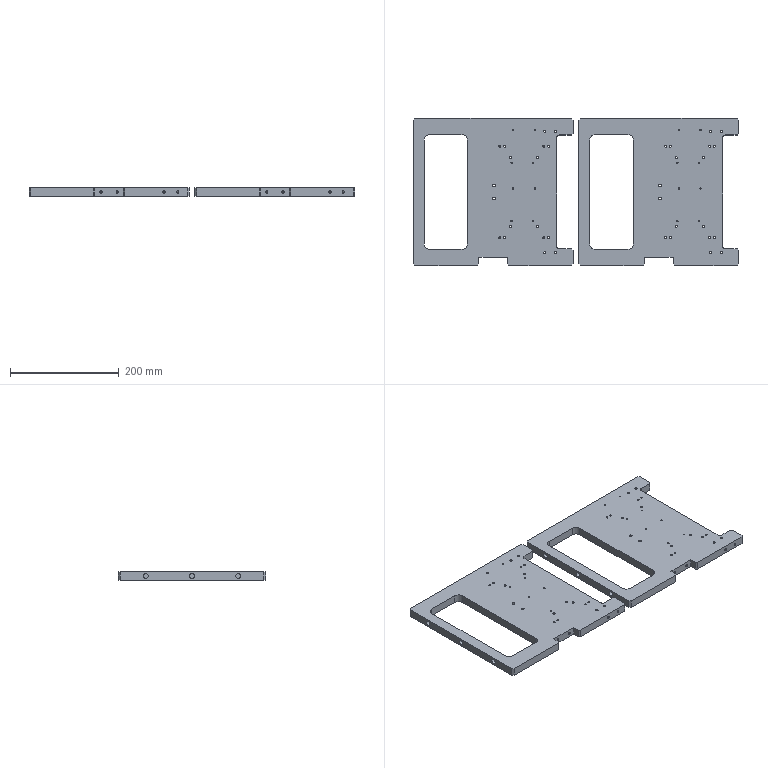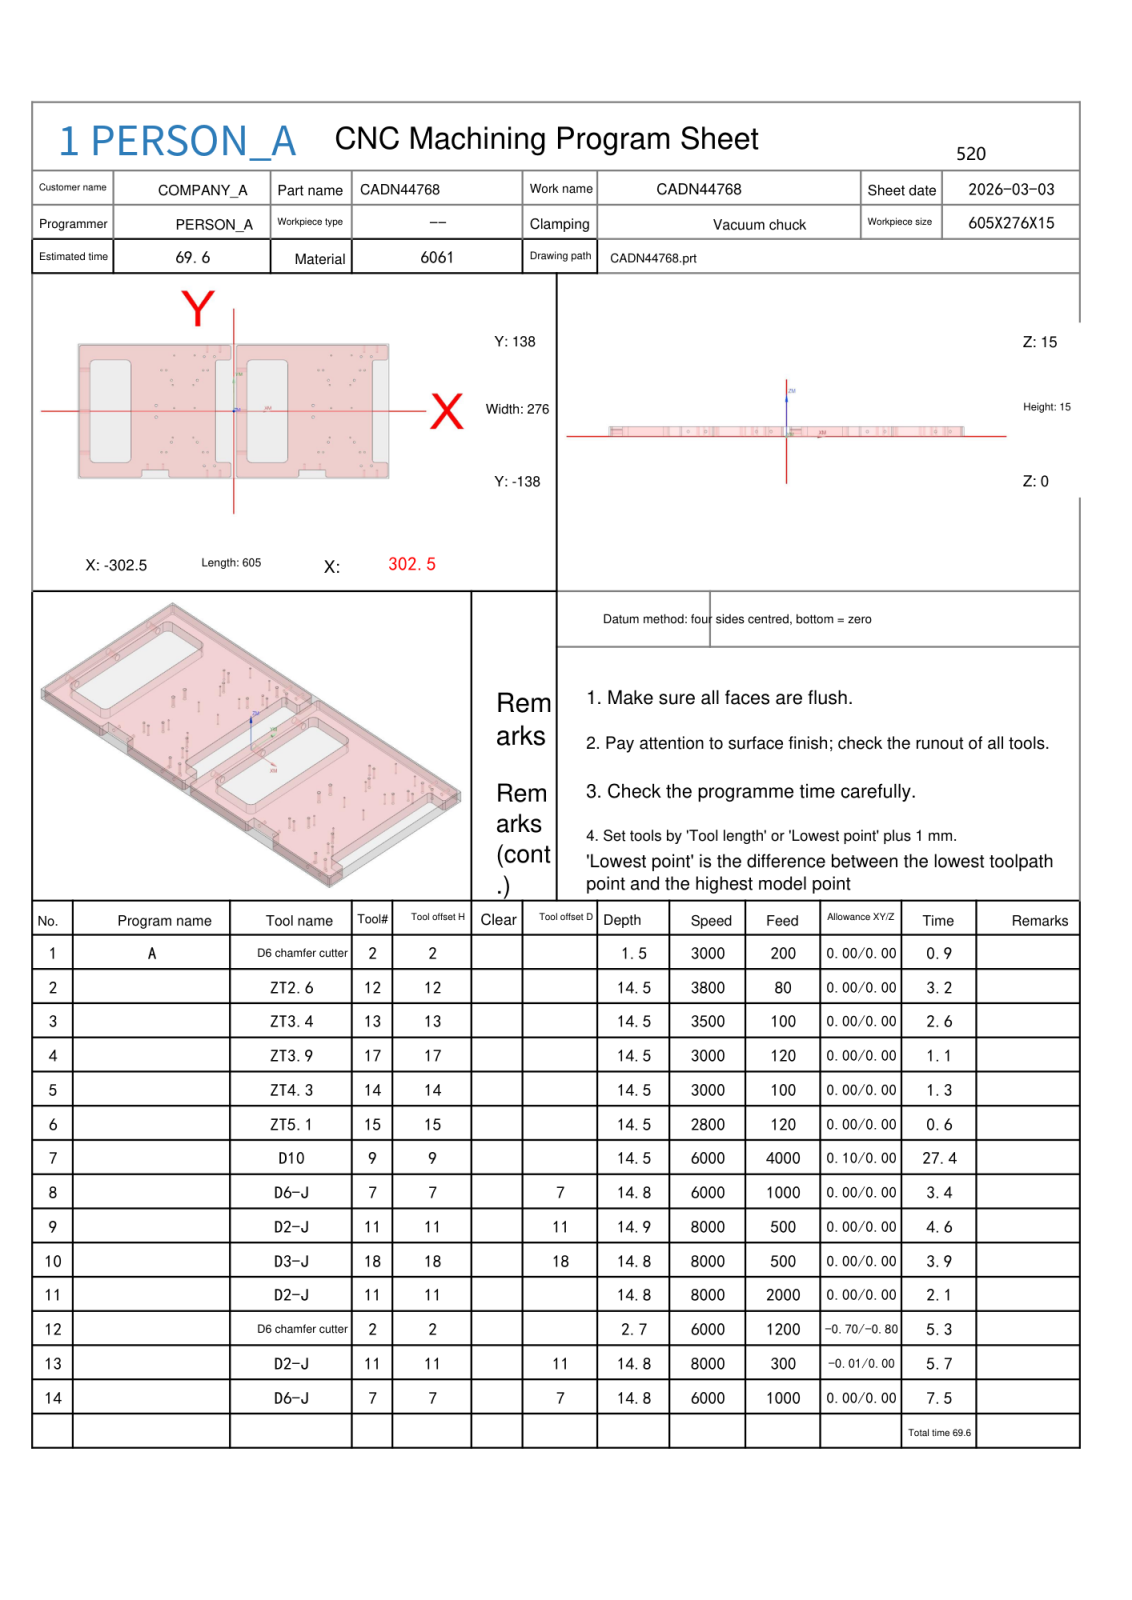NC program | NX | posted by the shop | part box 600 x 271 x 15 mm
Lines 3156 to 3997 of 17346:
N9 T11 M06
(D2-J  D=2. R=0. H=11 ce=0.00 di=0.00)
(D.N=11 MAX_Z=45. MIN_Z=0.15 Time=4.56M)
G00 G90 G54 X-50.369 Y83.4 M03 S8000
G43 H11 Z45.
M08
Z15.5
G01 X-50.227 Y83.443 Z15.492 F500.
X-50.061 Y83.561 Z15.482
X-49.943 Y83.727 Z15.471
X-49.884 Y83.921 Z15.46
Y84.079 Z15.452
X-49.939 Y84.265 Z15.442
X-50.049 Y84.426 Z15.432
X-50.203 Y84.545 Z15.421
X-50.386 Y84.61 Z15.411
X-50.579 Y84.616 Z15.401
X-50.773 Y84.557 Z15.39
X-50.939 Y84.439 Z15.38
X-51.057 Y84.273 Z15.369
X-51.116 Y84.079 Z15.358
Y83.921 Z15.35
X-51.057 Y83.727 Z15.34
X-50.939 Y83.561 Z15.329
X-50.773 Y83.443 Z15.318
X-50.579 Y83.384 Z15.308
X-50.421 Z15.299
X-50.227 Y83.443 Z15.289
X-50.061 Y83.561 Z15.278
X-49.943 Y83.727 Z15.267
X-49.884 Y83.921 Z15.257
Y84.079 Z15.248
X-49.939 Y84.265 Z15.238
X-50.049 Y84.426 Z15.228
X-50.203 Y84.545 Z15.218
X-50.386 Y84.61 Z15.208
X-50.579 Y84.616 Z15.198
X-50.773 Y84.557 Z15.187
X-50.939 Y84.439 Z15.176
X-51.057 Y84.273 Z15.166
X-51.116 Y84.079 Z15.155
Y83.921 Z15.147
X-51.057 Y83.727 Z15.136
X-50.939 Y83.561 Z15.125
X-50.773 Y83.443 Z15.115
X-50.579 Y83.384 Z15.104
X-50.421 Z15.096
X-50.227 Y83.443 Z15.085
X-50.061 Y83.561 Z15.074
X-49.943 Y83.727 Z15.064
X-49.884 Y83.921 Z15.053
Y84.079 Z15.045
X-49.939 Y84.265 Z15.035
X-50.049 Y84.426 Z15.025
X-50.203 Y84.545 Z15.014
X-50.386 Y84.61 Z15.004
X-50.465 Y84.615 Z15.
G41 D11
X-50.5 Y84.65
G03 X-51.15 Y84. Z14.876 I0.0 J-.65
X-50.5 Y83.35 Z14.753 I.65 J0.0
X-49.85 Y84. Z14.629 I0.0 J.65
X-50.5 Y84.65 Z14.505 I-.65 J0.0
X-51.15 Y84. Z14.381 I0.0 J-.65
X-50.5 Y83.35 Z14.258 I.65 J0.0
X-49.85 Y84. Z14.134 I0.0 J.65
X-50.5 Y84.65 Z14.01 I-.65 J0.0
X-51.15 Y84. Z13.886 I0.0 J-.65
X-50.5 Y83.35 Z13.763 I.65 J0.0
X-49.85 Y84. Z13.639 I0.0 J.65
X-50.5 Y84.65 Z13.515 I-.65 J0.0
X-51.15 Y84. Z13.391 I0.0 J-.65
X-50.5 Y83.35 Z13.268 I.65 J0.0
X-49.85 Y84. Z13.144 I0.0 J.65
X-50.5 Y84.65 Z13.02 I-.65 J0.0
X-51.15 Y84. Z12.896 I0.0 J-.65
X-50.5 Y83.35 Z12.773 I.65 J0.0
X-49.85 Y84. Z12.649 I0.0 J.65
X-50.5 Y84.65 Z12.525 I-.65 J0.0
X-51.15 Y84. Z12.401 I0.0 J-.65
X-50.5 Y83.35 Z12.278 I.65 J0.0
X-49.85 Y84. Z12.154 I0.0 J.65
X-50.5 Y84.65 Z12.03 I-.65 J0.0
X-51.15 Y84. Z11.906 I0.0 J-.65
X-50.5 Y83.35 Z11.783 I.65 J0.0
X-49.85 Y84. Z11.659 I0.0 J.65
X-50.5 Y84.65 Z11.535 I-.65 J0.0
X-51.15 Y84. Z11.411 I0.0 J-.65
X-50.5 Y83.35 Z11.288 I.65 J0.0
X-49.85 Y84. Z11.164 I0.0 J.65
X-50.5 Y84.65 Z11.04 I-.65 J0.0
X-51.15 Y84. Z10.916 I0.0 J-.65
X-50.5 Y83.35 Z10.793 I.65 J0.0
X-49.85 Y84. Z10.669 I0.0 J.65
X-50.5 Y84.65 Z10.545 I-.65 J0.0
X-51.15 Y84. Z10.421 I0.0 J-.65
X-50.5 Y83.35 Z10.298 I.65 J0.0
X-49.85 Y84. Z10.174 I0.0 J.65
X-50.5 Y84.65 Z10.05 I-.65 J0.0
X-51.15 Y84. Z9.926 I0.0 J-.65
X-50.5 Y83.35 Z9.803 I.65 J0.0
X-49.85 Y84. Z9.679 I0.0 J.65
X-50.5 Y84.65 Z9.555 I-.65 J0.0
X-51.15 Y84. Z9.431 I0.0 J-.65
X-50.5 Y83.35 Z9.308 I.65 J0.0
X-49.85 Y84. Z9.184 I0.0 J.65
X-50.5 Y84.65 Z9.06 I-.65 J0.0
X-51.15 Y84. Z8.936 I0.0 J-.65
X-50.5 Y83.35 Z8.813 I.65 J0.0
X-49.85 Y84. Z8.689 I0.0 J.65
X-50.5 Y84.65 Z8.565 I-.65 J0.0
X-51.15 Y84. Z8.441 I0.0 J-.65
X-50.5 Y83.35 Z8.318 I.65 J0.0
X-49.85 Y84. Z8.194 I0.0 J.65
X-50.5 Y84.65 Z8.07 I-.65 J0.0
X-51.15 Y84. Z7.946 I0.0 J-.65
X-50.5 Y83.35 Z7.823 I.65 J0.0
X-49.85 Y84. Z7.699 I0.0 J.65
X-50.5 Y84.65 Z7.575 I-.65 J0.0
X-51.15 Y84. Z7.451 I0.0 J-.65
X-50.5 Y83.35 Z7.328 I.65 J0.0
X-49.85 Y84. Z7.204 I0.0 J.65
X-50.5 Y84.65 Z7.08 I-.65 J0.0
X-51.15 Y84. Z6.956 I0.0 J-.65
X-50.5 Y83.35 Z6.833 I.65 J0.0
X-49.85 Y84. Z6.709 I0.0 J.65
X-50.5 Y84.65 Z6.585 I-.65 J0.0
X-51.15 Y84. Z6.461 I0.0 J-.65
X-50.5 Y83.35 Z6.338 I.65 J0.0
X-49.85 Y84. Z6.214 I0.0 J.65
X-50.5 Y84.65 Z6.09 I-.65 J0.0
X-51.15 Y84. Z5.966 I0.0 J-.65
X-50.5 Y83.35 Z5.843 I.65 J0.0
X-49.85 Y84. Z5.719 I0.0 J.65
X-50.5 Y84.65 Z5.595 I-.65 J0.0
X-51.15 Y84. Z5.471 I0.0 J-.65
X-50.5 Y83.35 Z5.348 I.65 J0.0
X-49.85 Y84. Z5.224 I0.0 J.65
X-50.5 Y84.65 Z5.1 I-.65 J0.0
X-51.15 Y84. Z4.976 I0.0 J-.65
X-50.5 Y83.35 Z4.853 I.65 J0.0
X-49.85 Y84. Z4.729 I0.0 J.65
X-50.5 Y84.65 Z4.605 I-.65 J0.0
X-51.15 Y84. Z4.481 I0.0 J-.65
X-50.5 Y83.35 Z4.358 I.65 J0.0
X-49.85 Y84. Z4.234 I0.0 J.65
X-50.5 Y84.65 Z4.11 I-.65 J0.0
X-51.15 Y84. Z3.986 I0.0 J-.65
X-50.5 Y83.35 Z3.863 I.65 J0.0
X-49.85 Y84. Z3.739 I0.0 J.65
X-50.5 Y84.65 Z3.615 I-.65 J0.0
X-51.15 Y84. Z3.491 I0.0 J-.65
X-50.5 Y83.35 Z3.368 I.65 J0.0
X-49.85 Y84. Z3.244 I0.0 J.65
X-50.5 Y84.65 Z3.12 I-.65 J0.0
X-51.15 Y84. Z2.996 I0.0 J-.65
X-50.5 Y83.35 Z2.873 I.65 J0.0
X-49.85 Y84. Z2.749 I0.0 J.65
X-50.5 Y84.65 Z2.625 I-.65 J0.0
X-51.15 Y84. Z2.501 I0.0 J-.65
X-50.5 Y83.35 Z2.378 I.65 J0.0
X-49.85 Y84. Z2.254 I0.0 J.65
X-50.5 Y84.65 Z2.13 I-.65 J0.0
X-51.15 Y84. Z2.006 I0.0 J-.65
X-50.5 Y83.35 Z1.883 I.65 J0.0
X-49.85 Y84. Z1.759 I0.0 J.65
X-50.5 Y84.65 Z1.635 I-.65 J0.0
X-51.15 Y84. Z1.511 I0.0 J-.65
X-50.5 Y83.35 Z1.388 I.65 J0.0
X-49.85 Y84. Z1.264 I0.0 J.65
X-50.5 Y84.65 Z1.14 I-.65 J0.0
X-51.15 Y84. Z1.016 I0.0 J-.65
X-50.5 Y83.35 Z.893 I.65 J0.0
X-49.85 Y84. Z.769 I0.0 J.65
X-50.5 Y84.65 Z.645 I-.65 J0.0
X-51.15 Y84. Z.521 I0.0 J-.65
X-50.5 Y83.35 Z.398 I.65 J0.0
X-49.85 Y84. Z.274 I0.0 J.65
X-50.5 Y84.65 Z.15 I-.65 J0.0
X-51.15 Y84. I0.0 J-.65
X-50.5 Y83.35 I.65 J0.0
X-49.85 Y84. I0.0 J.65
X-50.5 Y84.65 I-.65 J0.0
X-50.875 Y84.531 I0.0 J-.65
G01 X-50.896 Y84.513
X-50.901 Y84.485
X-50.887 Y84.461
G40 X-50.858 Y84.42
Z1.15
G00 Z45.
X-59.369 Y83.4
Z15.5
G01 X-59.227 Y83.443 Z15.492
X-59.061 Y83.561 Z15.482
X-58.943 Y83.727 Z15.471
X-58.884 Y83.921 Z15.46
Y84.079 Z15.452
X-58.939 Y84.265 Z15.442
X-59.049 Y84.426 Z15.432
X-59.203 Y84.545 Z15.421
X-59.386 Y84.61 Z15.411
X-59.579 Y84.616 Z15.401
X-59.773 Y84.557 Z15.39
X-59.939 Y84.439 Z15.38
X-60.057 Y84.273 Z15.369
X-60.116 Y84.079 Z15.358
Y83.921 Z15.35
X-60.057 Y83.727 Z15.34
X-59.939 Y83.561 Z15.329
X-59.773 Y83.443 Z15.318
X-59.579 Y83.384 Z15.308
X-59.421 Z15.299
X-59.227 Y83.443 Z15.289
X-59.061 Y83.561 Z15.278
X-58.943 Y83.727 Z15.267
X-58.884 Y83.921 Z15.257
Y84.079 Z15.248
X-58.939 Y84.265 Z15.238
X-59.049 Y84.426 Z15.228
X-59.203 Y84.545 Z15.218
X-59.386 Y84.61 Z15.208
X-59.579 Y84.616 Z15.198
X-59.773 Y84.557 Z15.187
X-59.939 Y84.439 Z15.176
X-60.057 Y84.273 Z15.166
X-60.116 Y84.079 Z15.155
Y83.921 Z15.147
X-60.057 Y83.727 Z15.136
X-59.939 Y83.561 Z15.125
X-59.773 Y83.443 Z15.115
X-59.579 Y83.384 Z15.104
X-59.421 Z15.096
X-59.227 Y83.443 Z15.085
X-59.061 Y83.561 Z15.074
X-58.943 Y83.727 Z15.064
X-58.884 Y83.921 Z15.053
Y84.079 Z15.045
X-58.939 Y84.265 Z15.035
X-59.049 Y84.426 Z15.025
X-59.203 Y84.545 Z15.014
X-59.386 Y84.61 Z15.004
X-59.465 Y84.615 Z15.
G41 D11
X-59.5 Y84.65
G03 X-60.15 Y84. Z14.876 I0.0 J-.65
X-59.5 Y83.35 Z14.753 I.65 J0.0
X-58.85 Y84. Z14.629 I0.0 J.65
X-59.5 Y84.65 Z14.505 I-.65 J0.0
X-60.15 Y84. Z14.381 I0.0 J-.65
X-59.5 Y83.35 Z14.258 I.65 J0.0
X-58.85 Y84. Z14.134 I0.0 J.65
X-59.5 Y84.65 Z14.01 I-.65 J0.0
X-60.15 Y84. Z13.886 I0.0 J-.65
X-59.5 Y83.35 Z13.763 I.65 J0.0
X-58.85 Y84. Z13.639 I0.0 J.65
X-59.5 Y84.65 Z13.515 I-.65 J0.0
X-60.15 Y84. Z13.391 I0.0 J-.65
X-59.5 Y83.35 Z13.268 I.65 J0.0
X-58.85 Y84. Z13.144 I0.0 J.65
X-59.5 Y84.65 Z13.02 I-.65 J0.0
X-60.15 Y84. Z12.896 I0.0 J-.65
X-59.5 Y83.35 Z12.773 I.65 J0.0
X-58.85 Y84. Z12.649 I0.0 J.65
X-59.5 Y84.65 Z12.525 I-.65 J0.0
X-60.15 Y84. Z12.401 I0.0 J-.65
X-59.5 Y83.35 Z12.278 I.65 J0.0
X-58.85 Y84. Z12.154 I0.0 J.65
X-59.5 Y84.65 Z12.03 I-.65 J0.0
X-60.15 Y84. Z11.906 I0.0 J-.65
X-59.5 Y83.35 Z11.783 I.65 J0.0
X-58.85 Y84. Z11.659 I0.0 J.65
X-59.5 Y84.65 Z11.535 I-.65 J0.0
X-60.15 Y84. Z11.411 I0.0 J-.65
X-59.5 Y83.35 Z11.288 I.65 J0.0
X-58.85 Y84. Z11.164 I0.0 J.65
X-59.5 Y84.65 Z11.04 I-.65 J0.0
X-60.15 Y84. Z10.916 I0.0 J-.65
X-59.5 Y83.35 Z10.793 I.65 J0.0
X-58.85 Y84. Z10.669 I0.0 J.65
X-59.5 Y84.65 Z10.545 I-.65 J0.0
X-60.15 Y84. Z10.421 I0.0 J-.65
X-59.5 Y83.35 Z10.298 I.65 J0.0
X-58.85 Y84. Z10.174 I0.0 J.65
X-59.5 Y84.65 Z10.05 I-.65 J0.0
X-60.15 Y84. Z9.926 I0.0 J-.65
X-59.5 Y83.35 Z9.803 I.65 J0.0
X-58.85 Y84. Z9.679 I0.0 J.65
X-59.5 Y84.65 Z9.555 I-.65 J0.0
X-60.15 Y84. Z9.431 I0.0 J-.65
X-59.5 Y83.35 Z9.308 I.65 J0.0
X-58.85 Y84. Z9.184 I0.0 J.65
X-59.5 Y84.65 Z9.06 I-.65 J0.0
X-60.15 Y84. Z8.936 I0.0 J-.65
X-59.5 Y83.35 Z8.813 I.65 J0.0
X-58.85 Y84. Z8.689 I0.0 J.65
X-59.5 Y84.65 Z8.565 I-.65 J0.0
X-60.15 Y84. Z8.441 I0.0 J-.65
X-59.5 Y83.35 Z8.318 I.65 J0.0
X-58.85 Y84. Z8.194 I0.0 J.65
X-59.5 Y84.65 Z8.07 I-.65 J0.0
X-60.15 Y84. Z7.946 I0.0 J-.65
X-59.5 Y83.35 Z7.823 I.65 J0.0
X-58.85 Y84. Z7.699 I0.0 J.65
X-59.5 Y84.65 Z7.575 I-.65 J0.0
X-60.15 Y84. Z7.451 I0.0 J-.65
X-59.5 Y83.35 Z7.328 I.65 J0.0
X-58.85 Y84. Z7.204 I0.0 J.65
X-59.5 Y84.65 Z7.08 I-.65 J0.0
X-60.15 Y84. Z6.956 I0.0 J-.65
X-59.5 Y83.35 Z6.833 I.65 J0.0
X-58.85 Y84. Z6.709 I0.0 J.65
X-59.5 Y84.65 Z6.585 I-.65 J0.0
X-60.15 Y84. Z6.461 I0.0 J-.65
X-59.5 Y83.35 Z6.338 I.65 J0.0
X-58.85 Y84. Z6.214 I0.0 J.65
X-59.5 Y84.65 Z6.09 I-.65 J0.0
X-60.15 Y84. Z5.966 I0.0 J-.65
X-59.5 Y83.35 Z5.843 I.65 J0.0
X-58.85 Y84. Z5.719 I0.0 J.65
X-59.5 Y84.65 Z5.595 I-.65 J0.0
X-60.15 Y84. Z5.471 I0.0 J-.65
X-59.5 Y83.35 Z5.348 I.65 J0.0
X-58.85 Y84. Z5.224 I0.0 J.65
X-59.5 Y84.65 Z5.1 I-.65 J0.0
X-60.15 Y84. Z4.976 I0.0 J-.65
X-59.5 Y83.35 Z4.853 I.65 J0.0
X-58.85 Y84. Z4.729 I0.0 J.65
X-59.5 Y84.65 Z4.605 I-.65 J0.0
X-60.15 Y84. Z4.481 I0.0 J-.65
X-59.5 Y83.35 Z4.358 I.65 J0.0
X-58.85 Y84. Z4.234 I0.0 J.65
X-59.5 Y84.65 Z4.11 I-.65 J0.0
X-60.15 Y84. Z3.986 I0.0 J-.65
X-59.5 Y83.35 Z3.863 I.65 J0.0
X-58.85 Y84. Z3.739 I0.0 J.65
X-59.5 Y84.65 Z3.615 I-.65 J0.0
X-60.15 Y84. Z3.491 I0.0 J-.65
X-59.5 Y83.35 Z3.368 I.65 J0.0
X-58.85 Y84. Z3.244 I0.0 J.65
X-59.5 Y84.65 Z3.12 I-.65 J0.0
X-60.15 Y84. Z2.996 I0.0 J-.65
X-59.5 Y83.35 Z2.873 I.65 J0.0
X-58.85 Y84. Z2.749 I0.0 J.65
X-59.5 Y84.65 Z2.625 I-.65 J0.0
X-60.15 Y84. Z2.501 I0.0 J-.65
X-59.5 Y83.35 Z2.378 I.65 J0.0
X-58.85 Y84. Z2.254 I0.0 J.65
X-59.5 Y84.65 Z2.13 I-.65 J0.0
X-60.15 Y84. Z2.006 I0.0 J-.65
X-59.5 Y83.35 Z1.883 I.65 J0.0
X-58.85 Y84. Z1.759 I0.0 J.65
X-59.5 Y84.65 Z1.635 I-.65 J0.0
X-60.15 Y84. Z1.511 I0.0 J-.65
X-59.5 Y83.35 Z1.388 I.65 J0.0
X-58.85 Y84. Z1.264 I0.0 J.65
X-59.5 Y84.65 Z1.14 I-.65 J0.0
X-60.15 Y84. Z1.016 I0.0 J-.65
X-59.5 Y83.35 Z.893 I.65 J0.0
X-58.85 Y84. Z.769 I0.0 J.65
X-59.5 Y84.65 Z.645 I-.65 J0.0
X-60.15 Y84. Z.521 I0.0 J-.65
X-59.5 Y83.35 Z.398 I.65 J0.0
X-58.85 Y84. Z.274 I0.0 J.65
X-59.5 Y84.65 Z.15 I-.65 J0.0
X-60.15 Y84. I0.0 J-.65
X-59.5 Y83.35 I.65 J0.0
X-58.85 Y84. I0.0 J.65
X-59.5 Y84.65 I-.65 J0.0
X-59.875 Y84.531 I0.0 J-.65
G01 X-59.896 Y84.513
X-59.901 Y84.485
X-59.887 Y84.461
G40 X-59.858 Y84.42
Z1.15
G00 Z45.
X-131.369 Y83.4
Z15.5
G01 X-131.227 Y83.443 Z15.492
X-131.061 Y83.561 Z15.482
X-130.943 Y83.727 Z15.471
X-130.884 Y83.921 Z15.46
Y84.079 Z15.452
X-130.939 Y84.265 Z15.442
X-131.049 Y84.426 Z15.432
X-131.203 Y84.545 Z15.421
X-131.386 Y84.61 Z15.411
X-131.579 Y84.616 Z15.401
X-131.773 Y84.557 Z15.39
X-131.939 Y84.439 Z15.38
X-132.057 Y84.273 Z15.369
X-132.116 Y84.079 Z15.358
Y83.921 Z15.35
X-132.057 Y83.727 Z15.34
X-131.939 Y83.561 Z15.329
X-131.773 Y83.443 Z15.318
X-131.579 Y83.384 Z15.308
X-131.421 Z15.299
X-131.227 Y83.443 Z15.289
X-131.061 Y83.561 Z15.278
X-130.943 Y83.727 Z15.267
X-130.884 Y83.921 Z15.257
Y84.079 Z15.248
X-130.939 Y84.265 Z15.238
X-131.049 Y84.426 Z15.228
X-131.203 Y84.545 Z15.218
X-131.386 Y84.61 Z15.208
X-131.579 Y84.616 Z15.198
X-131.773 Y84.557 Z15.187
X-131.939 Y84.439 Z15.176
X-132.057 Y84.273 Z15.166
X-132.116 Y84.079 Z15.155
Y83.921 Z15.147
X-132.057 Y83.727 Z15.136
X-131.939 Y83.561 Z15.125
X-131.773 Y83.443 Z15.115
X-131.579 Y83.384 Z15.104
X-131.421 Z15.096
X-131.227 Y83.443 Z15.085
X-131.061 Y83.561 Z15.074
X-130.943 Y83.727 Z15.064
X-130.884 Y83.921 Z15.053
Y84.079 Z15.045
X-130.939 Y84.265 Z15.035
X-131.049 Y84.426 Z15.025
X-131.203 Y84.545 Z15.014
X-131.386 Y84.61 Z15.004
X-131.465 Y84.615 Z15.
G41 D11
X-131.5 Y84.65
G03 X-132.15 Y84. Z14.876 I0.0 J-.65
X-131.5 Y83.35 Z14.753 I.65 J0.0
X-130.85 Y84. Z14.629 I0.0 J.65
X-131.5 Y84.65 Z14.505 I-.65 J0.0
X-132.15 Y84. Z14.381 I0.0 J-.65
X-131.5 Y83.35 Z14.258 I.65 J0.0
X-130.85 Y84. Z14.134 I0.0 J.65
X-131.5 Y84.65 Z14.01 I-.65 J0.0
X-132.15 Y84. Z13.886 I0.0 J-.65
X-131.5 Y83.35 Z13.763 I.65 J0.0
X-130.85 Y84. Z13.639 I0.0 J.65
X-131.5 Y84.65 Z13.515 I-.65 J0.0
X-132.15 Y84. Z13.391 I0.0 J-.65
X-131.5 Y83.35 Z13.268 I.65 J0.0
X-130.85 Y84. Z13.144 I0.0 J.65
X-131.5 Y84.65 Z13.02 I-.65 J0.0
X-132.15 Y84. Z12.896 I0.0 J-.65
X-131.5 Y83.35 Z12.773 I.65 J0.0
X-130.85 Y84. Z12.649 I0.0 J.65
X-131.5 Y84.65 Z12.525 I-.65 J0.0
X-132.15 Y84. Z12.401 I0.0 J-.65
X-131.5 Y83.35 Z12.278 I.65 J0.0
X-130.85 Y84. Z12.154 I0.0 J.65
X-131.5 Y84.65 Z12.03 I-.65 J0.0
X-132.15 Y84. Z11.906 I0.0 J-.65
X-131.5 Y83.35 Z11.783 I.65 J0.0
X-130.85 Y84. Z11.659 I0.0 J.65
X-131.5 Y84.65 Z11.535 I-.65 J0.0
X-132.15 Y84. Z11.411 I0.0 J-.65
X-131.5 Y83.35 Z11.288 I.65 J0.0
X-130.85 Y84. Z11.164 I0.0 J.65
X-131.5 Y84.65 Z11.04 I-.65 J0.0
X-132.15 Y84. Z10.916 I0.0 J-.65
X-131.5 Y83.35 Z10.793 I.65 J0.0
X-130.85 Y84. Z10.669 I0.0 J.65
X-131.5 Y84.65 Z10.545 I-.65 J0.0
X-132.15 Y84. Z10.421 I0.0 J-.65
X-131.5 Y83.35 Z10.298 I.65 J0.0
X-130.85 Y84. Z10.174 I0.0 J.65
X-131.5 Y84.65 Z10.05 I-.65 J0.0
X-132.15 Y84. Z9.926 I0.0 J-.65
X-131.5 Y83.35 Z9.803 I.65 J0.0
X-130.85 Y84. Z9.679 I0.0 J.65
X-131.5 Y84.65 Z9.555 I-.65 J0.0
X-132.15 Y84. Z9.431 I0.0 J-.65
X-131.5 Y83.35 Z9.308 I.65 J0.0
X-130.85 Y84. Z9.184 I0.0 J.65
X-131.5 Y84.65 Z9.06 I-.65 J0.0
X-132.15 Y84. Z8.936 I0.0 J-.65
X-131.5 Y83.35 Z8.813 I.65 J0.0
X-130.85 Y84. Z8.689 I0.0 J.65
X-131.5 Y84.65 Z8.565 I-.65 J0.0
X-132.15 Y84. Z8.441 I0.0 J-.65
X-131.5 Y83.35 Z8.318 I.65 J0.0
X-130.85 Y84. Z8.194 I0.0 J.65
X-131.5 Y84.65 Z8.07 I-.65 J0.0
X-132.15 Y84. Z7.946 I0.0 J-.65
X-131.5 Y83.35 Z7.823 I.65 J0.0
X-130.85 Y84. Z7.699 I0.0 J.65
X-131.5 Y84.65 Z7.575 I-.65 J0.0
X-132.15 Y84. Z7.451 I0.0 J-.65
X-131.5 Y83.35 Z7.328 I.65 J0.0
X-130.85 Y84. Z7.204 I0.0 J.65
X-131.5 Y84.65 Z7.08 I-.65 J0.0
X-132.15 Y84. Z6.956 I0.0 J-.65
X-131.5 Y83.35 Z6.833 I.65 J0.0
X-130.85 Y84. Z6.709 I0.0 J.65
X-131.5 Y84.65 Z6.585 I-.65 J0.0
X-132.15 Y84. Z6.461 I0.0 J-.65
X-131.5 Y83.35 Z6.338 I.65 J0.0
X-130.85 Y84. Z6.214 I0.0 J.65
X-131.5 Y84.65 Z6.09 I-.65 J0.0
X-132.15 Y84. Z5.966 I0.0 J-.65
X-131.5 Y83.35 Z5.843 I.65 J0.0
X-130.85 Y84. Z5.719 I0.0 J.65
X-131.5 Y84.65 Z5.595 I-.65 J0.0
X-132.15 Y84. Z5.471 I0.0 J-.65
X-131.5 Y83.35 Z5.348 I.65 J0.0
X-130.85 Y84. Z5.224 I0.0 J.65
X-131.5 Y84.65 Z5.1 I-.65 J0.0
X-132.15 Y84. Z4.976 I0.0 J-.65
X-131.5 Y83.35 Z4.853 I.65 J0.0
X-130.85 Y84. Z4.729 I0.0 J.65
X-131.5 Y84.65 Z4.605 I-.65 J0.0
X-132.15 Y84. Z4.481 I0.0 J-.65
X-131.5 Y83.35 Z4.358 I.65 J0.0
X-130.85 Y84. Z4.234 I0.0 J.65
X-131.5 Y84.65 Z4.11 I-.65 J0.0
X-132.15 Y84. Z3.986 I0.0 J-.65
X-131.5 Y83.35 Z3.863 I.65 J0.0
X-130.85 Y84. Z3.739 I0.0 J.65
X-131.5 Y84.65 Z3.615 I-.65 J0.0
X-132.15 Y84. Z3.491 I0.0 J-.65
X-131.5 Y83.35 Z3.368 I.65 J0.0
X-130.85 Y84. Z3.244 I0.0 J.65
X-131.5 Y84.65 Z3.12 I-.65 J0.0
X-132.15 Y84. Z2.996 I0.0 J-.65
X-131.5 Y83.35 Z2.873 I.65 J0.0
X-130.85 Y84. Z2.749 I0.0 J.65
X-131.5 Y84.65 Z2.625 I-.65 J0.0
X-132.15 Y84. Z2.501 I0.0 J-.65
X-131.5 Y83.35 Z2.378 I.65 J0.0
X-130.85 Y84. Z2.254 I0.0 J.65
X-131.5 Y84.65 Z2.13 I-.65 J0.0
X-132.15 Y84. Z2.006 I0.0 J-.65
X-131.5 Y83.35 Z1.883 I.65 J0.0
X-130.85 Y84. Z1.759 I0.0 J.65
X-131.5 Y84.65 Z1.635 I-.65 J0.0
X-132.15 Y84. Z1.511 I0.0 J-.65
X-131.5 Y83.35 Z1.388 I.65 J0.0
X-130.85 Y84. Z1.264 I0.0 J.65
X-131.5 Y84.65 Z1.14 I-.65 J0.0
X-132.15 Y84. Z1.016 I0.0 J-.65
X-131.5 Y83.35 Z.893 I.65 J0.0
X-130.85 Y84. Z.769 I0.0 J.65
X-131.5 Y84.65 Z.645 I-.65 J0.0
X-132.15 Y84. Z.521 I0.0 J-.65
X-131.5 Y83.35 Z.398 I.65 J0.0
X-130.85 Y84. Z.274 I0.0 J.65
X-131.5 Y84.65 Z.15 I-.65 J0.0
X-132.15 Y84. I0.0 J-.65
X-131.5 Y83.35 I.65 J0.0
X-130.85 Y84. I0.0 J.65
X-131.5 Y84.65 I-.65 J0.0
X-131.875 Y84.531 I0.0 J-.65
G01 X-131.896 Y84.513
X-131.901 Y84.485
X-131.887 Y84.461
G40 X-131.858 Y84.42
Z1.15
G00 Z45.
X-140.369 Y83.4
Z15.5
G01 X-140.227 Y83.443 Z15.492
X-140.061 Y83.561 Z15.482
X-139.943 Y83.727 Z15.471
X-139.884 Y83.921 Z15.46
Y84.079 Z15.452
X-139.939 Y84.265 Z15.442
X-140.049 Y84.426 Z15.432
X-140.203 Y84.545 Z15.421
X-140.386 Y84.61 Z15.411
X-140.579 Y84.616 Z15.401
X-140.773 Y84.557 Z15.39
X-140.939 Y84.439 Z15.38
X-141.057 Y84.273 Z15.369
X-141.116 Y84.079 Z15.358
Y83.921 Z15.35
X-141.057 Y83.727 Z15.34
X-140.939 Y83.561 Z15.329
X-140.773 Y83.443 Z15.318
X-140.579 Y83.384 Z15.308
X-140.421 Z15.299
X-140.227 Y83.443 Z15.289
X-140.061 Y83.561 Z15.278
X-139.943 Y83.727 Z15.267
X-139.884 Y83.921 Z15.257
Y84.079 Z15.248
X-139.939 Y84.265 Z15.238
X-140.049 Y84.426 Z15.228
X-140.203 Y84.545 Z15.218
X-140.386 Y84.61 Z15.208
X-140.579 Y84.616 Z15.198
X-140.773 Y84.557 Z15.187
X-140.939 Y84.439 Z15.176
X-141.057 Y84.273 Z15.166
X-141.116 Y84.079 Z15.155
Y83.921 Z15.147
X-141.057 Y83.727 Z15.136
X-140.939 Y83.561 Z15.125
X-140.773 Y83.443 Z15.115
X-140.579 Y83.384 Z15.104
X-140.421 Z15.096
X-140.227 Y83.443 Z15.085
X-140.061 Y83.561 Z15.074
X-139.943 Y83.727 Z15.064
X-139.884 Y83.921 Z15.053
Y84.079 Z15.045
X-139.939 Y84.265 Z15.035
X-140.049 Y84.426 Z15.025
X-140.203 Y84.545 Z15.014
X-140.386 Y84.61 Z15.004
X-140.465 Y84.615 Z15.
G41 D11
X-140.5 Y84.65
G03 X-141.15 Y84. Z14.876 I0.0 J-.65
X-140.5 Y83.35 Z14.753 I.65 J0.0
X-139.85 Y84. Z14.629 I0.0 J.65
X-140.5 Y84.65 Z14.505 I-.65 J0.0
X-141.15 Y84. Z14.381 I0.0 J-.65
X-140.5 Y83.35 Z14.258 I.65 J0.0
X-139.85 Y84. Z14.134 I0.0 J.65
X-140.5 Y84.65 Z14.01 I-.65 J0.0
X-141.15 Y84. Z13.886 I0.0 J-.65
X-140.5 Y83.35 Z13.763 I.65 J0.0
X-139.85 Y84. Z13.639 I0.0 J.65
X-140.5 Y84.65 Z13.515 I-.65 J0.0
X-141.15 Y84. Z13.391 I0.0 J-.65
X-140.5 Y83.35 Z13.268 I.65 J0.0
X-139.85 Y84. Z13.144 I0.0 J.65
X-140.5 Y84.65 Z13.02 I-.65 J0.0
X-141.15 Y84. Z12.896 I0.0 J-.65
X-140.5 Y83.35 Z12.773 I.65 J0.0
X-139.85 Y84. Z12.649 I0.0 J.65
X-140.5 Y84.65 Z12.525 I-.65 J0.0
X-141.15 Y84. Z12.401 I0.0 J-.65
X-140.5 Y83.35 Z12.278 I.65 J0.0
X-139.85 Y84. Z12.154 I0.0 J.65
X-140.5 Y84.65 Z12.03 I-.65 J0.0
X-141.15 Y84. Z11.906 I0.0 J-.65
X-140.5 Y83.35 Z11.783 I.65 J0.0
X-139.85 Y84. Z11.659 I0.0 J.65
X-140.5 Y84.65 Z11.535 I-.65 J0.0
X-141.15 Y84. Z11.411 I0.0 J-.65
X-140.5 Y83.35 Z11.288 I.65 J0.0
X-139.85 Y84. Z11.164 I0.0 J.65
X-140.5 Y84.65 Z11.04 I-.65 J0.0
X-141.15 Y84. Z10.916 I0.0 J-.65
X-140.5 Y83.35 Z10.793 I.65 J0.0
X-139.85 Y84. Z10.669 I0.0 J.65
X-140.5 Y84.65 Z10.545 I-.65 J0.0
X-141.15 Y84. Z10.421 I0.0 J-.65
X-140.5 Y83.35 Z10.298 I.65 J0.0
X-139.85 Y84. Z10.174 I0.0 J.65
X-140.5 Y84.65 Z10.05 I-.65 J0.0
X-141.15 Y84. Z9.926 I0.0 J-.65
X-140.5 Y83.35 Z9.803 I.65 J0.0
X-139.85 Y84. Z9.679 I0.0 J.65
X-140.5 Y84.65 Z9.555 I-.65 J0.0
X-141.15 Y84. Z9.431 I0.0 J-.65
X-140.5 Y83.35 Z9.308 I.65 J0.0
X-139.85 Y84. Z9.184 I0.0 J.65
X-140.5 Y84.65 Z9.06 I-.65 J0.0
X-141.15 Y84. Z8.936 I0.0 J-.65
X-140.5 Y83.35 Z8.813 I.65 J0.0
X-139.85 Y84. Z8.689 I0.0 J.65
X-140.5 Y84.65 Z8.565 I-.65 J0.0
X-141.15 Y84. Z8.441 I0.0 J-.65
X-140.5 Y83.35 Z8.318 I.65 J0.0
X-139.85 Y84. Z8.194 I0.0 J.65
X-140.5 Y84.65 Z8.07 I-.65 J0.0
X-141.15 Y84. Z7.946 I0.0 J-.65
X-140.5 Y83.35 Z7.823 I.65 J0.0
X-139.85 Y84. Z7.699 I0.0 J.65
X-140.5 Y84.65 Z7.575 I-.65 J0.0
X-141.15 Y84. Z7.451 I0.0 J-.65
X-140.5 Y83.35 Z7.328 I.65 J0.0
X-139.85 Y84. Z7.204 I0.0 J.65
X-140.5 Y84.65 Z7.08 I-.65 J0.0
X-141.15 Y84. Z6.956 I0.0 J-.65
X-140.5 Y83.35 Z6.833 I.65 J0.0
X-139.85 Y84. Z6.709 I0.0 J.65
X-140.5 Y84.65 Z6.585 I-.65 J0.0
X-141.15 Y84. Z6.461 I0.0 J-.65
X-140.5 Y83.35 Z6.338 I.65 J0.0
X-139.85 Y84. Z6.214 I0.0 J.65
X-140.5 Y84.65 Z6.09 I-.65 J0.0
X-141.15 Y84. Z5.966 I0.0 J-.65
X-140.5 Y83.35 Z5.843 I.65 J0.0
X-139.85 Y84. Z5.719 I0.0 J.65
X-140.5 Y84.65 Z5.595 I-.65 J0.0
X-141.15 Y84. Z5.471 I0.0 J-.65
X-140.5 Y83.35 Z5.348 I.65 J0.0
X-139.85 Y84. Z5.224 I0.0 J.65
X-140.5 Y84.65 Z5.1 I-.65 J0.0
X-141.15 Y84. Z4.976 I0.0 J-.65
X-140.5 Y83.35 Z4.853 I.65 J0.0
X-139.85 Y84. Z4.729 I0.0 J.65
X-140.5 Y84.65 Z4.605 I-.65 J0.0
X-141.15 Y84. Z4.481 I0.0 J-.65
X-140.5 Y83.35 Z4.358 I.65 J0.0
X-139.85 Y84. Z4.234 I0.0 J.65
X-140.5 Y84.65 Z4.11 I-.65 J0.0
X-141.15 Y84. Z3.986 I0.0 J-.65
X-140.5 Y83.35 Z3.863 I.65 J0.0
X-139.85 Y84. Z3.739 I0.0 J.65
X-140.5 Y84.65 Z3.615 I-.65 J0.0
X-141.15 Y84. Z3.491 I0.0 J-.65
X-140.5 Y83.35 Z3.368 I.65 J0.0
X-139.85 Y84. Z3.244 I0.0 J.65
X-140.5 Y84.65 Z3.12 I-.65 J0.0
X-141.15 Y84. Z2.996 I0.0 J-.65
X-140.5 Y83.35 Z2.873 I.65 J0.0
X-139.85 Y84. Z2.749 I0.0 J.65
X-140.5 Y84.65 Z2.625 I-.65 J0.0
X-141.15 Y84. Z2.501 I0.0 J-.65
X-140.5 Y83.35 Z2.378 I.65 J0.0
X-139.85 Y84. Z2.254 I0.0 J.65
X-140.5 Y84.65 Z2.13 I-.65 J0.0
X-141.15 Y84. Z2.006 I0.0 J-.65
X-140.5 Y83.35 Z1.883 I.65 J0.0
X-139.85 Y84. Z1.759 I0.0 J.65
X-140.5 Y84.65 Z1.635 I-.65 J0.0
X-141.15 Y84. Z1.511 I0.0 J-.65
X-140.5 Y83.35 Z1.388 I.65 J0.0
X-139.85 Y84. Z1.264 I0.0 J.65
X-140.5 Y84.65 Z1.14 I-.65 J0.0
X-141.15 Y84. Z1.016 I0.0 J-.65
X-140.5 Y83.35 Z.893 I.65 J0.0
X-139.85 Y84. Z.769 I0.0 J.65
X-140.5 Y84.65 Z.645 I-.65 J0.0
X-141.15 Y84. Z.521 I0.0 J-.65
X-140.5 Y83.35 Z.398 I.65 J0.0
X-139.85 Y84. Z.274 I0.0 J.65
X-140.5 Y84.65 Z.15 I-.65 J0.0
X-141.15 Y84. I0.0 J-.65
X-140.5 Y83.35 I.65 J0.0
X-139.85 Y84. I0.0 J.65
X-140.5 Y84.65 I-.65 J0.0
X-140.875 Y84.531 I0.0 J-.65
G01 X-140.896 Y84.513
X-140.901 Y84.485
X-140.887 Y84.461
G40 X-140.858 Y84.42
Z1.15
G00 Z45.
X-140.631 Y-83.4
Z15.5
G01 X-140.773 Y-83.443 Z15.492
X-140.939 Y-83.561 Z15.482
X-141.057 Y-83.727 Z15.471
X-141.116 Y-83.921 Z15.46
Y-84.079 Z15.452
X-141.061 Y-84.265 Z15.442
X-140.951 Y-84.426 Z15.432
X-140.797 Y-84.545 Z15.421
X-140.614 Y-84.61 Z15.411
X-140.421 Y-84.616 Z15.401
X-140.227 Y-84.557 Z15.39
X-140.061 Y-84.439 Z15.38
X-139.943 Y-84.273 Z15.369
X-139.884 Y-84.079 Z15.358
Y-83.921 Z15.35
X-139.943 Y-83.727 Z15.34
X-140.061 Y-83.561 Z15.329
X-140.227 Y-83.443 Z15.318
X-140.421 Y-83.384 Z15.308
X-140.579 Z15.299
X-140.773 Y-83.443 Z15.289
X-140.939 Y-83.561 Z15.278
X-141.057 Y-83.727 Z15.267
X-141.116 Y-83.921 Z15.257
Y-84.079 Z15.248
X-141.061 Y-84.265 Z15.238
X-140.951 Y-84.426 Z15.228
X-140.797 Y-84.545 Z15.218
X-140.614 Y-84.61 Z15.208
X-140.421 Y-84.616 Z15.198
X-140.227 Y-84.557 Z15.187
X-140.061 Y-84.439 Z15.176
X-139.943 Y-84.273 Z15.166
X-139.884 Y-84.079 Z15.155
Y-83.921 Z15.147
X-139.943 Y-83.727 Z15.136
X-140.061 Y-83.561 Z15.125
X-140.227 Y-83.443 Z15.115
X-140.421 Y-83.384 Z15.104
X-140.579 Z15.096
X-140.773 Y-83.443 Z15.085
X-140.939 Y-83.561 Z15.074
X-141.057 Y-83.727 Z15.064
X-141.116 Y-83.921 Z15.053
Y-84.079 Z15.045
X-141.061 Y-84.265 Z15.035
X-140.951 Y-84.426 Z15.025
X-140.797 Y-84.545 Z15.014
X-140.614 Y-84.61 Z15.004
X-140.535 Y-84.615 Z15.
G41 D11
X-140.5 Y-84.65
G03 X-139.85 Y-84. Z14.876 I0.0 J.65
X-140.5 Y-83.35 Z14.753 I-.65 J0.0
X-141.15 Y-84. Z14.629 I0.0 J-.65
X-140.5 Y-84.65 Z14.505 I.65 J0.0
X-139.85 Y-84. Z14.381 I0.0 J.65
X-140.5 Y-83.35 Z14.258 I-.65 J0.0
X-141.15 Y-84. Z14.134 I0.0 J-.65
X-140.5 Y-84.65 Z14.01 I.65 J0.0
X-139.85 Y-84. Z13.886 I0.0 J.65
X-140.5 Y-83.35 Z13.763 I-.65 J0.0
X-141.15 Y-84. Z13.639 I0.0 J-.65
X-140.5 Y-84.65 Z13.515 I.65 J0.0
X-139.85 Y-84. Z13.391 I0.0 J.65
X-140.5 Y-83.35 Z13.268 I-.65 J0.0
X-141.15 Y-84. Z13.144 I0.0 J-.65
X-140.5 Y-84.65 Z13.02 I.65 J0.0
X-139.85 Y-84. Z12.896 I0.0 J.65
X-140.5 Y-83.35 Z12.773 I-.65 J0.0
X-141.15 Y-84. Z12.649 I0.0 J-.65
X-140.5 Y-84.65 Z12.525 I.65 J0.0
X-139.85 Y-84. Z12.401 I0.0 J.65
X-140.5 Y-83.35 Z12.278 I-.65 J0.0
X-141.15 Y-84. Z12.154 I0.0 J-.65
X-140.5 Y-84.65 Z12.03 I.65 J0.0
X-139.85 Y-84. Z11.906 I0.0 J.65
X-140.5 Y-83.35 Z11.783 I-.65 J0.0
X-141.15 Y-84. Z11.659 I0.0 J-.65
X-140.5 Y-84.65 Z11.535 I.65 J0.0
X-139.85 Y-84. Z11.411 I0.0 J.65
X-140.5 Y-83.35 Z11.288 I-.65 J0.0
X-141.15 Y-84. Z11.164 I0.0 J-.65
X-140.5 Y-84.65 Z11.04 I.65 J0.0
X-139.85 Y-84. Z10.916 I0.0 J.65
X-140.5 Y-83.35 Z10.793 I-.65 J0.0
X-141.15 Y-84. Z10.669 I0.0 J-.65
X-140.5 Y-84.65 Z10.545 I.65 J0.0
X-139.85 Y-84. Z10.421 I0.0 J.65
X-140.5 Y-83.35 Z10.298 I-.65 J0.0
X-141.15 Y-84. Z10.174 I0.0 J-.65
X-140.5 Y-84.65 Z10.05 I.65 J0.0
X-139.85 Y-84. Z9.926 I0.0 J.65
X-140.5 Y-83.35 Z9.803 I-.65 J0.0
X-141.15 Y-84. Z9.679 I0.0 J-.65